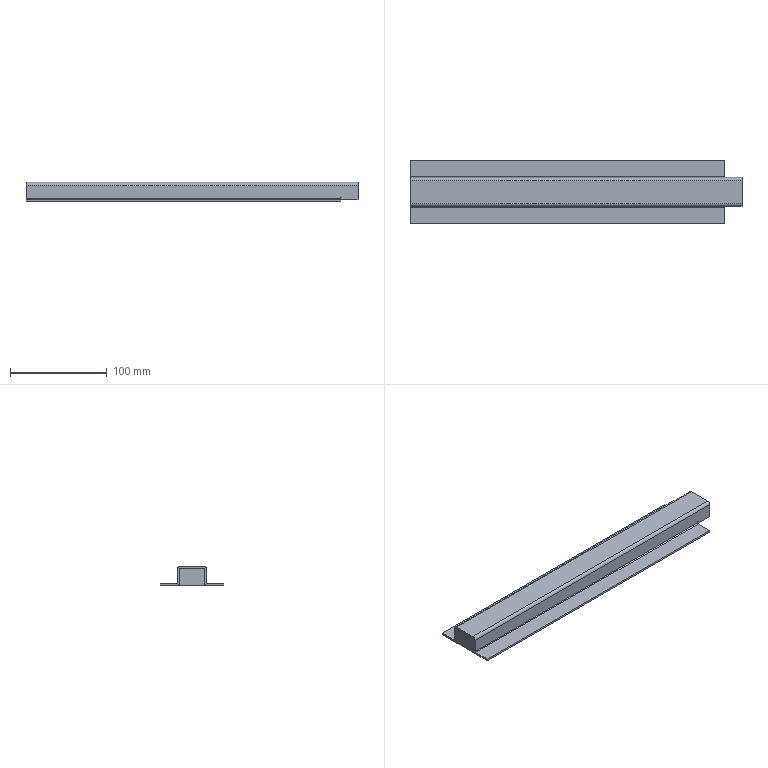Part | SolidWorks | features BaseBody 2 | 2 solids | 56 faces | box 343.5 x 66 x 20 mm | volume 67264 mm3 | plane 46 | cylinder 10 | commonest cylinder face diameters 2 x6 6 x4
STEP:
#1=CARTESIAN_POINT('',(154.75,15.,-18.));
#2=VERTEX_POINT('',#1);
#3=CARTESIAN_POINT('',(171.75,15.,-18.));
#4=VERTEX_POINT('',#3);
#5=CARTESIAN_POINT('',(0.,15.,-18.));
#6=DIRECTION('',(1.,0.,0.));
#7=VECTOR('',#6,1000.);
#8=LINE('',#5,#7);
#9=EDGE_CURVE('',#2,#4,#8,.T.);
#10=ORIENTED_EDGE('',*,*,#9,.T.);
#11=CARTESIAN_POINT('',(171.75,13.,-18.));
#12=VERTEX_POINT('',#11);
#13=CARTESIAN_POINT('',(171.75,33.,-18.));
#14=DIRECTION('',(0.,-1.,0.));
#15=VECTOR('',#14,1000.);
#16=LINE('',#13,#15);
#17=EDGE_CURVE('',#4,#12,#16,.T.);
#18=ORIENTED_EDGE('',*,*,#17,.T.);
#19=CARTESIAN_POINT('',(154.75,13.,-18.));
#20=VERTEX_POINT('',#19);
#21=CARTESIAN_POINT('',(0.,13.,-18.));
#22=DIRECTION('',(1.,0.,0.));
#23=VECTOR('',#22,1000.);
#24=LINE('',#21,#23);
#25=EDGE_CURVE('',#20,#12,#24,.T.);
#26=ORIENTED_EDGE('',*,*,#25,.F.);
#27=CARTESIAN_POINT('',(154.75,15.,-18.));
#28=DIRECTION('',(0.,1.,0.));
#29=VECTOR('',#28,1000.);
#30=LINE('',#27,#29);
#31=EDGE_CURVE('',#20,#2,#30,.T.);
#32=ORIENTED_EDGE('',*,*,#31,.T.);
#33=EDGE_LOOP('',(#10,#18,#26,#32));
#34=FACE_OUTER_BOUND('',#33,.T.);
#35=CARTESIAN_POINT('',(171.75,33.,-18.));
#36=DIRECTION('',(0.,0.,1.));
#37=DIRECTION('',(0.,-1.,0.));
#38=AXIS2_PLACEMENT_3D('',#35,#36,#37);
#39=PLANE('',#38);
#40=ADVANCED_FACE('',(#34),#39,.F.);
#41=CARTESIAN_POINT('',(154.75,-13.,-18.));
#42=VERTEX_POINT('',#41);
#43=CARTESIAN_POINT('',(171.75,-13.,-18.));
#44=VERTEX_POINT('',#43);
#45=CARTESIAN_POINT('',(0.,-13.,-18.));
#46=DIRECTION('',(1.,0.,0.));
#47=VECTOR('',#46,1000.);
#48=LINE('',#45,#47);
#49=EDGE_CURVE('',#42,#44,#48,.T.);
#50=ORIENTED_EDGE('',*,*,#49,.T.);
#51=CARTESIAN_POINT('',(171.75,-15.,-18.));
#52=VERTEX_POINT('',#51);
#53=CARTESIAN_POINT('',(171.75,33.,-18.));
#54=DIRECTION('',(0.,-1.,0.));
#55=VECTOR('',#54,1000.);
#56=LINE('',#53,#55);
#57=EDGE_CURVE('',#44,#52,#56,.T.);
#58=ORIENTED_EDGE('',*,*,#57,.T.);
#59=CARTESIAN_POINT('',(154.75,-15.,-18.));
#60=VERTEX_POINT('',#59);
#61=CARTESIAN_POINT('',(171.75,-15.,-18.));
#62=DIRECTION('',(-1.,0.,0.));
#63=VECTOR('',#62,1000.);
#64=LINE('',#61,#63);
#65=EDGE_CURVE('',#52,#60,#64,.T.);
#66=ORIENTED_EDGE('',*,*,#65,.T.);
#67=CARTESIAN_POINT('',(154.75,-15.,-18.));
#68=DIRECTION('',(0.,1.,0.));
#69=VECTOR('',#68,1000.);
#70=LINE('',#67,#69);
#71=EDGE_CURVE('',#60,#42,#70,.T.);
#72=ORIENTED_EDGE('',*,*,#71,.T.);
#73=EDGE_LOOP('',(#50,#58,#66,#72));
#74=FACE_OUTER_BOUND('',#73,.T.);
#75=CARTESIAN_POINT('',(171.75,33.,-18.));
#76=DIRECTION('',(0.,0.,1.));
#77=DIRECTION('',(0.,-1.,0.));
#78=AXIS2_PLACEMENT_3D('',#75,#76,#77);
#79=PLANE('',#78);
#80=ADVANCED_FACE('',(#74),#79,.F.);
#81=CARTESIAN_POINT('',(-171.75,-33.,-18.));
#82=VERTEX_POINT('',#81);
#83=CARTESIAN_POINT('',(153.75,-33.,-18.));
#84=VERTEX_POINT('',#83);
#85=CARTESIAN_POINT('',(0.,-33.,-18.));
#86=DIRECTION('',(1.,0.,0.));
#87=VECTOR('',#86,1000.);
#88=LINE('',#85,#87);
#89=EDGE_CURVE('',#82,#84,#88,.T.);
#90=ORIENTED_EDGE('',*,*,#89,.F.);
#91=CARTESIAN_POINT('',(-171.75,-33.,-20.));
#92=VERTEX_POINT('',#91);
#93=CARTESIAN_POINT('',(-171.75,-33.,-20.));
#94=DIRECTION('',(0.,0.,1.));
#95=VECTOR('',#94,1000.);
#96=LINE('',#93,#95);
#97=EDGE_CURVE('',#92,#82,#96,.T.);
#98=ORIENTED_EDGE('',*,*,#97,.F.);
#99=CARTESIAN_POINT('',(153.75,-33.,-20.));
#100=VERTEX_POINT('',#99);
#101=CARTESIAN_POINT('',(-171.75,-33.,-20.));
#102=DIRECTION('',(1.,0.,0.));
#103=VECTOR('',#102,1000.);
#104=LINE('',#101,#103);
#105=EDGE_CURVE('',#92,#100,#104,.T.);
#106=ORIENTED_EDGE('',*,*,#105,.T.);
#107=CARTESIAN_POINT('',(153.75,-33.,-20.));
#108=DIRECTION('',(0.,0.,1.));
#109=VECTOR('',#108,1000.);
#110=LINE('',#107,#109);
#111=EDGE_CURVE('',#100,#84,#110,.T.);
#112=ORIENTED_EDGE('',*,*,#111,.T.);
#113=EDGE_LOOP('',(#90,#98,#106,#112));
#114=FACE_OUTER_BOUND('',#113,.T.);
#115=CARTESIAN_POINT('',(-171.75,-33.,-20.));
#116=DIRECTION('',(0.,-1.,0.));
#117=DIRECTION('',(0.,0.,-1.));
#118=AXIS2_PLACEMENT_3D('',#115,#116,#117);
#119=PLANE('',#118);
#120=ADVANCED_FACE('',(#114),#119,.T.);
#121=CARTESIAN_POINT('',(153.75,-16.,-18.));
#122=VERTEX_POINT('',#121);
#123=CARTESIAN_POINT('',(153.75,0.,-18.));
#124=DIRECTION('',(0.,1.,0.));
#125=VECTOR('',#124,1000.);
#126=LINE('',#123,#125);
#127=EDGE_CURVE('',#84,#122,#126,.T.);
#128=ORIENTED_EDGE('',*,*,#127,.T.);
#129=CARTESIAN_POINT('',(-171.75,-16.,-18.));
#130=VERTEX_POINT('',#129);
#131=CARTESIAN_POINT('',(-171.75,-16.,-18.));
#132=DIRECTION('',(1.,0.,0.));
#133=VECTOR('',#132,1000.);
#134=LINE('',#131,#133);
#135=EDGE_CURVE('',#130,#122,#134,.T.);
#136=ORIENTED_EDGE('',*,*,#135,.F.);
#137=CARTESIAN_POINT('',(-171.75,0.,-18.));
#138=DIRECTION('',(0.,-1.,0.));
#139=VECTOR('',#138,1000.);
#140=LINE('',#137,#139);
#141=EDGE_CURVE('',#130,#82,#140,.T.);
#142=ORIENTED_EDGE('',*,*,#141,.T.);
#143=ORIENTED_EDGE('',*,*,#89,.T.);
#144=EDGE_LOOP('',(#128,#136,#142,#143));
#145=FACE_OUTER_BOUND('',#144,.T.);
#146=CARTESIAN_POINT('',(0.,0.,-18.));
#147=DIRECTION('',(0.,0.,1.));
#148=DIRECTION('',(1.,0.,0.));
#149=AXIS2_PLACEMENT_3D('',#146,#147,#148);
#150=PLANE('',#149);
#151=ADVANCED_FACE('',(#145),#150,.T.);
#152=CARTESIAN_POINT('',(153.75,-16.,-20.));
#153=VERTEX_POINT('',#152);
#154=CARTESIAN_POINT('',(-171.75,-16.,-20.));
#155=VERTEX_POINT('',#154);
#156=CARTESIAN_POINT('',(-171.75,-16.,-20.));
#157=DIRECTION('',(-1.,0.,0.));
#158=VECTOR('',#157,1000.);
#159=LINE('',#156,#158);
#160=EDGE_CURVE('',#153,#155,#159,.T.);
#161=ORIENTED_EDGE('',*,*,#160,.F.);
#162=CARTESIAN_POINT('',(153.75,-33.,-20.));
#163=DIRECTION('',(0.,1.,0.));
#164=VECTOR('',#163,1000.);
#165=LINE('',#162,#164);
#166=EDGE_CURVE('',#100,#153,#165,.T.);
#167=ORIENTED_EDGE('',*,*,#166,.F.);
#168=ORIENTED_EDGE('',*,*,#105,.F.);
#169=CARTESIAN_POINT('',(-171.75,-15.,-20.));
#170=DIRECTION('',(0.,-1.,0.));
#171=VECTOR('',#170,1000.);
#172=LINE('',#169,#171);
#173=EDGE_CURVE('',#155,#92,#172,.T.);
#174=ORIENTED_EDGE('',*,*,#173,.F.);
#175=EDGE_LOOP('',(#161,#167,#168,#174));
#176=FACE_OUTER_BOUND('',#175,.T.);
#177=CARTESIAN_POINT('',(0.,0.,-20.));
#178=DIRECTION('',(0.,0.,1.));
#179=DIRECTION('',(1.,0.,0.));
#180=AXIS2_PLACEMENT_3D('',#177,#178,#179);
#181=PLANE('',#180);
#182=ADVANCED_FACE('',(#176),#181,.F.);
#183=ORIENTED_EDGE('',*,*,#166,.T.);
#184=CARTESIAN_POINT('',(153.75,-16.,-18.));
#185=DIRECTION('',(0.,0.,-1.));
#186=VECTOR('',#185,1000.);
#187=LINE('',#184,#186);
#188=EDGE_CURVE('',#122,#153,#187,.T.);
#189=ORIENTED_EDGE('',*,*,#188,.F.);
#190=ORIENTED_EDGE('',*,*,#127,.F.);
#191=ORIENTED_EDGE('',*,*,#111,.F.);
#192=EDGE_LOOP('',(#183,#189,#190,#191));
#193=FACE_OUTER_BOUND('',#192,.T.);
#194=CARTESIAN_POINT('',(153.75,-33.,-20.));
#195=DIRECTION('',(1.,0.,0.));
#196=DIRECTION('',(0.,0.,-1.));
#197=AXIS2_PLACEMENT_3D('',#194,#195,#196);
#198=PLANE('',#197);
#199=ADVANCED_FACE('',(#193),#198,.T.);
#200=ORIENTED_EDGE('',*,*,#141,.F.);
#201=CARTESIAN_POINT('',(-171.75,-16.,-20.));
#202=DIRECTION('',(0.,0.,-1.));
#203=VECTOR('',#202,1000.);
#204=LINE('',#201,#203);
#205=EDGE_CURVE('',#130,#155,#204,.T.);
#206=ORIENTED_EDGE('',*,*,#205,.T.);
#207=ORIENTED_EDGE('',*,*,#173,.T.);
#208=ORIENTED_EDGE('',*,*,#97,.T.);
#209=EDGE_LOOP('',(#200,#206,#207,#208));
#210=FACE_OUTER_BOUND('',#209,.T.);
#211=CARTESIAN_POINT('',(-171.75,-15.,-20.));
#212=DIRECTION('',(-1.,0.,0.));
#213=DIRECTION('',(0.,1.,0.));
#214=AXIS2_PLACEMENT_3D('',#211,#212,#213);
#215=PLANE('',#214);
#216=ADVANCED_FACE('',(#210),#215,.T.);
#217=CARTESIAN_POINT('',(153.75,-15.,-17.));
#218=VERTEX_POINT('',#217);
#219=CARTESIAN_POINT('',(-171.75,-15.,-17.));
#220=VERTEX_POINT('',#219);
#221=CARTESIAN_POINT('',(153.75,-15.,-17.));
#222=DIRECTION('',(-1.,0.,0.));
#223=VECTOR('',#222,1000.);
#224=LINE('',#221,#223);
#225=EDGE_CURVE('',#218,#220,#224,.T.);
#226=ORIENTED_EDGE('',*,*,#225,.T.);
#227=CARTESIAN_POINT('',(-171.75,-16.,-17.));
#228=DIRECTION('',(-1.,0.,0.));
#229=DIRECTION('',(0.,0.,-1.));
#230=AXIS2_PLACEMENT_3D('',#227,#228,#229);
#231=CIRCLE('',#230,1.);
#232=EDGE_CURVE('',#220,#130,#231,.T.);
#233=ORIENTED_EDGE('',*,*,#232,.T.);
#234=ORIENTED_EDGE('',*,*,#135,.T.);
#235=CARTESIAN_POINT('',(153.75,-16.,-17.));
#236=DIRECTION('',(1.,0.,0.));
#237=DIRECTION('',(0.,0.,-1.));
#238=AXIS2_PLACEMENT_3D('',#235,#236,#237);
#239=CIRCLE('',#238,1.);
#240=EDGE_CURVE('',#122,#218,#239,.T.);
#241=ORIENTED_EDGE('',*,*,#240,.T.);
#242=EDGE_LOOP('',(#226,#233,#234,#241));
#243=FACE_OUTER_BOUND('',#242,.T.);
#244=CARTESIAN_POINT('',(153.75,-16.,-17.));
#245=DIRECTION('',(1.,0.,0.));
#246=DIRECTION('',(0.,0.,-1.));
#247=AXIS2_PLACEMENT_3D('',#244,#245,#246);
#248=CYLINDRICAL_SURFACE('',#247,1.);
#249=ADVANCED_FACE('',(#243),#248,.F.);
#250=CARTESIAN_POINT('',(153.75,-13.,-17.));
#251=VERTEX_POINT('',#250);
#252=CARTESIAN_POINT('',(-171.75,-13.,-17.));
#253=VERTEX_POINT('',#252);
#254=CARTESIAN_POINT('',(153.75,-13.,-17.));
#255=DIRECTION('',(-1.,0.,0.));
#256=VECTOR('',#255,1000.);
#257=LINE('',#254,#256);
#258=EDGE_CURVE('',#251,#253,#257,.T.);
#259=ORIENTED_EDGE('',*,*,#258,.F.);
#260=CARTESIAN_POINT('',(153.75,-13.172,-18.));
#261=VERTEX_POINT('',#260);
#262=CARTESIAN_POINT('',(153.75,-16.,-17.));
#263=DIRECTION('',(1.,0.,0.));
#264=DIRECTION('',(0.,0.,-1.));
#265=AXIS2_PLACEMENT_3D('',#262,#263,#264);
#266=CIRCLE('',#265,3.);
#267=EDGE_CURVE('',#261,#251,#266,.T.);
#268=ORIENTED_EDGE('',*,*,#267,.F.);
#269=CARTESIAN_POINT('',(153.75,-15.,-19.828));
#270=VERTEX_POINT('',#269);
#271=CARTESIAN_POINT('',(153.75,-16.,-17.));
#272=DIRECTION('',(1.,0.,0.));
#273=DIRECTION('',(0.,0.,-1.));
#274=AXIS2_PLACEMENT_3D('',#271,#272,#273);
#275=CIRCLE('',#274,3.);
#276=EDGE_CURVE('',#270,#261,#275,.T.);
#277=ORIENTED_EDGE('',*,*,#276,.F.);
#278=CARTESIAN_POINT('',(153.75,-16.,-17.));
#279=DIRECTION('',(1.,0.,0.));
#280=DIRECTION('',(0.,0.,-1.));
#281=AXIS2_PLACEMENT_3D('',#278,#279,#280);
#282=CIRCLE('',#281,3.);
#283=EDGE_CURVE('',#153,#270,#282,.T.);
#284=ORIENTED_EDGE('',*,*,#283,.F.);
#285=ORIENTED_EDGE('',*,*,#160,.T.);
#286=CARTESIAN_POINT('',(-171.75,-16.,-17.));
#287=DIRECTION('',(-1.,0.,0.));
#288=DIRECTION('',(0.,0.,-1.));
#289=AXIS2_PLACEMENT_3D('',#286,#287,#288);
#290=CIRCLE('',#289,3.);
#291=EDGE_CURVE('',#253,#155,#290,.T.);
#292=ORIENTED_EDGE('',*,*,#291,.F.);
#293=EDGE_LOOP('',(#259,#268,#277,#284,#285,#292));
#294=FACE_OUTER_BOUND('',#293,.T.);
#295=CARTESIAN_POINT('',(153.75,-16.,-17.));
#296=DIRECTION('',(1.,0.,0.));
#297=DIRECTION('',(0.,0.,-1.));
#298=AXIS2_PLACEMENT_3D('',#295,#296,#297);
#299=CYLINDRICAL_SURFACE('',#298,3.);
#300=ADVANCED_FACE('',(#294),#299,.T.);
#301=CARTESIAN_POINT('',(153.75,-15.,-18.));
#302=VERTEX_POINT('',#301);
#303=CARTESIAN_POINT('',(153.75,-16.,-18.));
#304=DIRECTION('',(0.,-1.,0.));
#305=VECTOR('',#304,1000.);
#306=LINE('',#303,#305);
#307=EDGE_CURVE('',#261,#302,#306,.T.);
#308=ORIENTED_EDGE('',*,*,#307,.F.);
#309=ORIENTED_EDGE('',*,*,#267,.T.);
#310=CARTESIAN_POINT('',(153.75,-15.,-17.));
#311=DIRECTION('',(0.,1.,0.));
#312=VECTOR('',#311,1000.);
#313=LINE('',#310,#312);
#314=EDGE_CURVE('',#218,#251,#313,.T.);
#315=ORIENTED_EDGE('',*,*,#314,.F.);
#316=ORIENTED_EDGE('',*,*,#240,.F.);
#317=ORIENTED_EDGE('',*,*,#188,.T.);
#318=ORIENTED_EDGE('',*,*,#283,.T.);
#319=CARTESIAN_POINT('',(153.75,-15.,-17.));
#320=DIRECTION('',(0.,0.,-1.));
#321=VECTOR('',#320,1000.);
#322=LINE('',#319,#321);
#323=EDGE_CURVE('',#302,#270,#322,.T.);
#324=ORIENTED_EDGE('',*,*,#323,.F.);
#325=EDGE_LOOP('',(#308,#309,#315,#316,#317,#318,#324));
#326=FACE_OUTER_BOUND('',#325,.T.);
#327=CARTESIAN_POINT('',(153.75,-16.,-17.));
#328=DIRECTION('',(-1.,0.,0.));
#329=DIRECTION('',(0.,0.,1.));
#330=AXIS2_PLACEMENT_3D('',#327,#328,#329);
#331=PLANE('',#330);
#332=ADVANCED_FACE('',(#326),#331,.F.);
#333=ORIENTED_EDGE('',*,*,#205,.F.);
#334=ORIENTED_EDGE('',*,*,#232,.F.);
#335=CARTESIAN_POINT('',(-171.75,-15.,-17.));
#336=DIRECTION('',(0.,1.,0.));
#337=VECTOR('',#336,1000.);
#338=LINE('',#335,#337);
#339=EDGE_CURVE('',#220,#253,#338,.T.);
#340=ORIENTED_EDGE('',*,*,#339,.T.);
#341=ORIENTED_EDGE('',*,*,#291,.T.);
#342=EDGE_LOOP('',(#333,#334,#340,#341));
#343=FACE_OUTER_BOUND('',#342,.T.);
#344=CARTESIAN_POINT('',(-171.75,-16.,-17.));
#345=DIRECTION('',(-1.,0.,0.));
#346=DIRECTION('',(0.,0.,1.));
#347=AXIS2_PLACEMENT_3D('',#344,#345,#346);
#348=PLANE('',#347);
#349=ADVANCED_FACE('',(#343),#348,.T.);
#350=CARTESIAN_POINT('',(153.75,33.,-18.));
#351=VERTEX_POINT('',#350);
#352=CARTESIAN_POINT('',(-171.75,33.,-18.));
#353=VERTEX_POINT('',#352);
#354=CARTESIAN_POINT('',(0.,33.,-18.));
#355=DIRECTION('',(-1.,0.,0.));
#356=VECTOR('',#355,1000.);
#357=LINE('',#354,#356);
#358=EDGE_CURVE('',#351,#353,#357,.T.);
#359=ORIENTED_EDGE('',*,*,#358,.F.);
#360=CARTESIAN_POINT('',(153.75,33.,-20.));
#361=VERTEX_POINT('',#360);
#362=CARTESIAN_POINT('',(153.75,33.,-20.));
#363=DIRECTION('',(0.,0.,1.));
#364=VECTOR('',#363,1000.);
#365=LINE('',#362,#364);
#366=EDGE_CURVE('',#361,#351,#365,.T.);
#367=ORIENTED_EDGE('',*,*,#366,.F.);
#368=CARTESIAN_POINT('',(-171.75,33.,-20.));
#369=VERTEX_POINT('',#368);
#370=CARTESIAN_POINT('',(-171.75,33.,-20.));
#371=DIRECTION('',(-1.,0.,0.));
#372=VECTOR('',#371,1000.);
#373=LINE('',#370,#372);
#374=EDGE_CURVE('',#361,#369,#373,.T.);
#375=ORIENTED_EDGE('',*,*,#374,.T.);
#376=CARTESIAN_POINT('',(-171.75,33.,-20.));
#377=DIRECTION('',(0.,0.,1.));
#378=VECTOR('',#377,1000.);
#379=LINE('',#376,#378);
#380=EDGE_CURVE('',#369,#353,#379,.T.);
#381=ORIENTED_EDGE('',*,*,#380,.T.);
#382=EDGE_LOOP('',(#359,#367,#375,#381));
#383=FACE_OUTER_BOUND('',#382,.T.);
#384=CARTESIAN_POINT('',(-171.75,33.,-20.));
#385=DIRECTION('',(0.,1.,0.));
#386=DIRECTION('',(1.,0.,0.));
#387=AXIS2_PLACEMENT_3D('',#384,#385,#386);
#388=PLANE('',#387);
#389=ADVANCED_FACE('',(#383),#388,.T.);
#390=CARTESIAN_POINT('',(153.75,16.,-18.));
#391=VERTEX_POINT('',#390);
#392=CARTESIAN_POINT('',(-171.75,16.,-18.));
#393=VERTEX_POINT('',#392);
#394=CARTESIAN_POINT('',(153.75,16.,-18.));
#395=DIRECTION('',(-1.,0.,0.));
#396=VECTOR('',#395,1000.);
#397=LINE('',#394,#396);
#398=EDGE_CURVE('',#391,#393,#397,.T.);
#399=ORIENTED_EDGE('',*,*,#398,.F.);
#400=CARTESIAN_POINT('',(153.75,0.,-18.));
#401=DIRECTION('',(0.,1.,0.));
#402=VECTOR('',#401,1000.);
#403=LINE('',#400,#402);
#404=EDGE_CURVE('',#391,#351,#403,.T.);
#405=ORIENTED_EDGE('',*,*,#404,.T.);
#406=ORIENTED_EDGE('',*,*,#358,.T.);
#407=CARTESIAN_POINT('',(-171.75,0.,-18.));
#408=DIRECTION('',(0.,-1.,0.));
#409=VECTOR('',#408,1000.);
#410=LINE('',#407,#409);
#411=EDGE_CURVE('',#353,#393,#410,.T.);
#412=ORIENTED_EDGE('',*,*,#411,.T.);
#413=EDGE_LOOP('',(#399,#405,#406,#412));
#414=FACE_OUTER_BOUND('',#413,.T.);
#415=CARTESIAN_POINT('',(0.,0.,-18.));
#416=DIRECTION('',(0.,0.,-1.));
#417=DIRECTION('',(0.,-1.,0.));
#418=AXIS2_PLACEMENT_3D('',#415,#416,#417);
#419=PLANE('',#418);
#420=ADVANCED_FACE('',(#414),#419,.F.);
#421=CARTESIAN_POINT('',(153.75,16.,-20.));
#422=VERTEX_POINT('',#421);
#423=CARTESIAN_POINT('',(153.75,15.,-20.));
#424=DIRECTION('',(0.,1.,0.));
#425=VECTOR('',#424,1000.);
#426=LINE('',#423,#425);
#427=EDGE_CURVE('',#422,#361,#426,.T.);
#428=ORIENTED_EDGE('',*,*,#427,.F.);
#429=CARTESIAN_POINT('',(-171.75,16.,-20.));
#430=VERTEX_POINT('',#429);
#431=CARTESIAN_POINT('',(0.,16.,-20.));
#432=DIRECTION('',(-1.,0.,0.));
#433=VECTOR('',#432,1000.);
#434=LINE('',#431,#433);
#435=EDGE_CURVE('',#422,#430,#434,.T.);
#436=ORIENTED_EDGE('',*,*,#435,.T.);
#437=CARTESIAN_POINT('',(-171.75,15.,-20.));
#438=DIRECTION('',(0.,-1.,0.));
#439=VECTOR('',#438,1000.);
#440=LINE('',#437,#439);
#441=EDGE_CURVE('',#369,#430,#440,.T.);
#442=ORIENTED_EDGE('',*,*,#441,.F.);
#443=ORIENTED_EDGE('',*,*,#374,.F.);
#444=EDGE_LOOP('',(#428,#436,#442,#443));
#445=FACE_OUTER_BOUND('',#444,.T.);
#446=CARTESIAN_POINT('',(0.,0.,-20.));
#447=DIRECTION('',(0.,0.,-1.));
#448=DIRECTION('',(0.,-1.,0.));
#449=AXIS2_PLACEMENT_3D('',#446,#447,#448);
#450=PLANE('',#449);
#451=ADVANCED_FACE('',(#445),#450,.T.);
#452=ORIENTED_EDGE('',*,*,#441,.T.);
#453=CARTESIAN_POINT('',(-171.75,16.,-18.));
#454=DIRECTION('',(0.,0.,-1.));
#455=VECTOR('',#454,1000.);
#456=LINE('',#453,#455);
#457=EDGE_CURVE('',#393,#430,#456,.T.);
#458=ORIENTED_EDGE('',*,*,#457,.F.);
#459=ORIENTED_EDGE('',*,*,#411,.F.);
#460=ORIENTED_EDGE('',*,*,#380,.F.);
#461=EDGE_LOOP('',(#452,#458,#459,#460));
#462=FACE_OUTER_BOUND('',#461,.T.);
#463=CARTESIAN_POINT('',(-171.75,15.,-20.));
#464=DIRECTION('',(-1.,0.,0.));
#465=DIRECTION('',(0.,0.,1.));
#466=AXIS2_PLACEMENT_3D('',#463,#464,#465);
#467=PLANE('',#466);
#468=ADVANCED_FACE('',(#462),#467,.T.);
#469=ORIENTED_EDGE('',*,*,#404,.F.);
#470=CARTESIAN_POINT('',(153.75,16.,-20.));
#471=DIRECTION('',(0.,0.,-1.));
#472=VECTOR('',#471,1000.);
#473=LINE('',#470,#472);
#474=EDGE_CURVE('',#391,#422,#473,.T.);
#475=ORIENTED_EDGE('',*,*,#474,.T.);
#476=ORIENTED_EDGE('',*,*,#427,.T.);
#477=ORIENTED_EDGE('',*,*,#366,.T.);
#478=EDGE_LOOP('',(#469,#475,#476,#477));
#479=FACE_OUTER_BOUND('',#478,.T.);
#480=CARTESIAN_POINT('',(153.75,15.,-20.));
#481=DIRECTION('',(1.,0.,0.));
#482=DIRECTION('',(0.,1.,0.));
#483=AXIS2_PLACEMENT_3D('',#480,#481,#482);
#484=PLANE('',#483);
#485=ADVANCED_FACE('',(#479),#484,.T.);
#486=CARTESIAN_POINT('',(-171.75,15.,-17.));
#487=VERTEX_POINT('',#486);
#488=CARTESIAN_POINT('',(153.75,15.,-17.));
#489=VERTEX_POINT('',#488);
#490=CARTESIAN_POINT('',(-171.75,15.,-17.));
#491=DIRECTION('',(1.,0.,0.));
#492=VECTOR('',#491,1000.);
#493=LINE('',#490,#492);
#494=EDGE_CURVE('',#487,#489,#493,.T.);
#495=ORIENTED_EDGE('',*,*,#494,.T.);
#496=CARTESIAN_POINT('',(153.75,16.,-17.));
#497=DIRECTION('',(1.,0.,0.));
#498=DIRECTION('',(0.,0.,1.));
#499=AXIS2_PLACEMENT_3D('',#496,#497,#498);
#500=CIRCLE('',#499,1.);
#501=EDGE_CURVE('',#489,#391,#500,.T.);
#502=ORIENTED_EDGE('',*,*,#501,.T.);
#503=ORIENTED_EDGE('',*,*,#398,.T.);
#504=CARTESIAN_POINT('',(-171.75,16.,-17.));
#505=DIRECTION('',(-1.,0.,0.));
#506=DIRECTION('',(0.,0.,1.));
#507=AXIS2_PLACEMENT_3D('',#504,#505,#506);
#508=CIRCLE('',#507,1.);
#509=EDGE_CURVE('',#393,#487,#508,.T.);
#510=ORIENTED_EDGE('',*,*,#509,.T.);
#511=EDGE_LOOP('',(#495,#502,#503,#510));
#512=FACE_OUTER_BOUND('',#511,.T.);
#513=CARTESIAN_POINT('',(-171.75,16.,-17.));
#514=DIRECTION('',(-1.,0.,0.));
#515=DIRECTION('',(0.,0.,-1.));
#516=AXIS2_PLACEMENT_3D('',#513,#514,#515);
#517=CYLINDRICAL_SURFACE('',#516,1.);
#518=ADVANCED_FACE('',(#512),#517,.F.);
#519=CARTESIAN_POINT('',(-171.75,13.,-17.));
#520=VERTEX_POINT('',#519);
#521=CARTESIAN_POINT('',(153.75,13.,-17.));
#522=VERTEX_POINT('',#521);
#523=CARTESIAN_POINT('',(-171.75,13.,-17.));
#524=DIRECTION('',(1.,0.,0.));
#525=VECTOR('',#524,1000.);
#526=LINE('',#523,#525);
#527=EDGE_CURVE('',#520,#522,#526,.T.);
#528=ORIENTED_EDGE('',*,*,#527,.F.);
#529=CARTESIAN_POINT('',(-171.75,16.,-17.));
#530=DIRECTION('',(-1.,0.,0.));
#531=DIRECTION('',(0.,0.,1.));
#532=AXIS2_PLACEMENT_3D('',#529,#530,#531);
#533=CIRCLE('',#532,3.);
#534=EDGE_CURVE('',#430,#520,#533,.T.);
#535=ORIENTED_EDGE('',*,*,#534,.F.);
#536=ORIENTED_EDGE('',*,*,#435,.F.);
#537=CARTESIAN_POINT('',(153.75,13.172,-18.));
#538=VERTEX_POINT('',#537);
#539=CARTESIAN_POINT('',(153.75,16.,-17.));
#540=DIRECTION('',(1.,0.,0.));
#541=DIRECTION('',(0.,0.,1.));
#542=AXIS2_PLACEMENT_3D('',#539,#540,#541);
#543=CIRCLE('',#542,3.);
#544=EDGE_CURVE('',#538,#422,#543,.T.);
#545=ORIENTED_EDGE('',*,*,#544,.F.);
#546=CARTESIAN_POINT('',(153.75,16.,-17.));
#547=DIRECTION('',(1.,0.,0.));
#548=DIRECTION('',(0.,0.,1.));
#549=AXIS2_PLACEMENT_3D('',#546,#547,#548);
#550=CIRCLE('',#549,3.);
#551=EDGE_CURVE('',#522,#538,#550,.T.);
#552=ORIENTED_EDGE('',*,*,#551,.F.);
#553=EDGE_LOOP('',(#528,#535,#536,#545,#552));
#554=FACE_OUTER_BOUND('',#553,.T.);
#555=CARTESIAN_POINT('',(-171.75,16.,-17.));
#556=DIRECTION('',(-1.,0.,0.));
#557=DIRECTION('',(0.,0.,-1.));
#558=AXIS2_PLACEMENT_3D('',#555,#556,#557);
#559=CYLINDRICAL_SURFACE('',#558,3.);
#560=ADVANCED_FACE('',(#554),#559,.T.);
#561=ORIENTED_EDGE('',*,*,#509,.F.);
#562=ORIENTED_EDGE('',*,*,#457,.T.);
#563=ORIENTED_EDGE('',*,*,#534,.T.);
#564=CARTESIAN_POINT('',(-171.75,15.,-17.));
#565=DIRECTION('',(0.,-1.,0.));
#566=VECTOR('',#565,1000.);
#567=LINE('',#564,#566);
#568=EDGE_CURVE('',#487,#520,#567,.T.);
#569=ORIENTED_EDGE('',*,*,#568,.F.);
#570=EDGE_LOOP('',(#561,#562,#563,#569));
#571=FACE_OUTER_BOUND('',#570,.T.);
#572=CARTESIAN_POINT('',(-171.75,16.,-17.));
#573=DIRECTION('',(1.,0.,0.));
#574=DIRECTION('',(0.,1.,0.));
#575=AXIS2_PLACEMENT_3D('',#572,#573,#574);
#576=PLANE('',#575);
#577=ADVANCED_FACE('',(#571),#576,.F.);
#578=CARTESIAN_POINT('',(153.75,16.,-18.));
#579=DIRECTION('',(0.,-1.,0.));
#580=VECTOR('',#579,1000.);
#581=LINE('',#578,#580);
#582=EDGE_CURVE('',#391,#538,#581,.T.);
#583=ORIENTED_EDGE('',*,*,#582,.F.);
#584=ORIENTED_EDGE('',*,*,#501,.F.);
#585=CARTESIAN_POINT('',(153.75,15.,-17.));
#586=DIRECTION('',(0.,-1.,0.));
#587=VECTOR('',#586,1000.);
#588=LINE('',#585,#587);
#589=EDGE_CURVE('',#489,#522,#588,.T.);
#590=ORIENTED_EDGE('',*,*,#589,.T.);
#591=ORIENTED_EDGE('',*,*,#551,.T.);
#592=EDGE_LOOP('',(#583,#584,#590,#591));
#593=FACE_OUTER_BOUND('',#592,.T.);
#594=CARTESIAN_POINT('',(153.75,16.,-17.));
#595=DIRECTION('',(1.,0.,0.));
#596=DIRECTION('',(0.,1.,0.));
#597=AXIS2_PLACEMENT_3D('',#594,#595,#596);
#598=PLANE('',#597);
#599=ADVANCED_FACE('',(#593),#598,.T.);
#600=CARTESIAN_POINT('',(153.75,-13.,-16.));
#601=VERTEX_POINT('',#600);
#602=CARTESIAN_POINT('',(153.75,-13.,0.));
#603=DIRECTION('',(0.,0.,-1.));
#604=VECTOR('',#603,1000.);
#605=LINE('',#602,#604);
#606=EDGE_CURVE('',#601,#251,#605,.T.);
#607=ORIENTED_EDGE('',*,*,#606,.F.);
#608=CARTESIAN_POINT('',(153.75,-15.,-16.));
#609=VERTEX_POINT('',#608);
#610=CARTESIAN_POINT('',(153.75,-15.,-16.));
#611=DIRECTION('',(0.,1.,0.));
#612=VECTOR('',#611,1000.);
#613=LINE('',#610,#612);
#614=EDGE_CURVE('',#609,#601,#613,.T.);
#615=ORIENTED_EDGE('',*,*,#614,.F.);
#616=CARTESIAN_POINT('',(153.75,-15.,-16.));
#617=DIRECTION('',(0.,0.,-1.));
#618=VECTOR('',#617,1000.);
#619=LINE('',#616,#618);
#620=EDGE_CURVE('',#609,#218,#619,.T.);
#621=ORIENTED_EDGE('',*,*,#620,.T.);
#622=ORIENTED_EDGE('',*,*,#314,.T.);
#623=EDGE_LOOP('',(#607,#615,#621,#622));
#624=FACE_OUTER_BOUND('',#623,.T.);
#625=CARTESIAN_POINT('',(153.75,-15.,-16.));
#626=DIRECTION('',(1.,0.,0.));
#627=DIRECTION('',(0.,1.,0.));
#628=AXIS2_PLACEMENT_3D('',#625,#626,#627);
#629=PLANE('',#628);
#630=ADVANCED_FACE('',(#624),#629,.T.);
#631=CARTESIAN_POINT('',(154.75,-13.,-16.));
#632=VERTEX_POINT('',#631);
#633=CARTESIAN_POINT('',(0.,-13.,-16.));
#634=DIRECTION('',(-1.,0.,0.));
#635=VECTOR('',#634,1000.);
#636=LINE('',#633,#635);
#637=EDGE_CURVE('',#632,#601,#636,.T.);
#638=ORIENTED_EDGE('',*,*,#637,.F.);
#639=CARTESIAN_POINT('',(154.75,-15.,-16.));
#640=VERTEX_POINT('',#639);
#641=CARTESIAN_POINT('',(154.75,-15.,-16.));
#642=DIRECTION('',(0.,1.,0.));
#643=VECTOR('',#642,1000.);
#644=LINE('',#641,#643);
#645=EDGE_CURVE('',#640,#632,#644,.T.);
#646=ORIENTED_EDGE('',*,*,#645,.F.);
#647=CARTESIAN_POINT('',(154.75,-15.,-16.));
#648=DIRECTION('',(-1.,0.,0.));
#649=VECTOR('',#648,1000.);
#650=LINE('',#647,#649);
#651=EDGE_CURVE('',#640,#609,#650,.T.);
#652=ORIENTED_EDGE('',*,*,#651,.T.);
#653=ORIENTED_EDGE('',*,*,#614,.T.);
#654=EDGE_LOOP('',(#638,#646,#652,#653));
#655=FACE_OUTER_BOUND('',#654,.T.);
#656=CARTESIAN_POINT('',(154.75,-15.,-16.));
#657=DIRECTION('',(0.,0.,-1.));
#658=DIRECTION('',(0.,-1.,0.));
#659=AXIS2_PLACEMENT_3D('',#656,#657,#658);
#660=PLANE('',#659);
#661=ADVANCED_FACE('',(#655),#660,.T.);
#662=ORIENTED_EDGE('',*,*,#71,.F.);
#663=CARTESIAN_POINT('',(154.75,-15.,-20.));
#664=DIRECTION('',(0.,0.,1.));
#665=VECTOR('',#664,1000.);
#666=LINE('',#663,#665);
#667=EDGE_CURVE('',#60,#640,#666,.T.);
#668=ORIENTED_EDGE('',*,*,#667,.T.);
#669=ORIENTED_EDGE('',*,*,#645,.T.);
#670=CARTESIAN_POINT('',(154.75,-13.,0.));
#671=DIRECTION('',(0.,0.,1.));
#672=VECTOR('',#671,1000.);
#673=LINE('',#670,#672);
#674=EDGE_CURVE('',#42,#632,#673,.T.);
#675=ORIENTED_EDGE('',*,*,#674,.F.);
#676=EDGE_LOOP('',(#662,#668,#669,#675));
#677=FACE_OUTER_BOUND('',#676,.T.);
#678=CARTESIAN_POINT('',(154.75,-15.,-20.));
#679=DIRECTION('',(-1.,0.,0.));
#680=DIRECTION('',(0.,1.,0.));
#681=AXIS2_PLACEMENT_3D('',#678,#679,#680);
#682=PLANE('',#681);
#683=ADVANCED_FACE('',(#677),#682,.T.);
#684=ORIENTED_EDGE('',*,*,#31,.F.);
#685=CARTESIAN_POINT('',(154.75,13.,-16.));
#686=VERTEX_POINT('',#685);
#687=CARTESIAN_POINT('',(154.75,13.,0.));
#688=DIRECTION('',(0.,0.,1.));
#689=VECTOR('',#688,1000.);
#690=LINE('',#687,#689);
#691=EDGE_CURVE('',#20,#686,#690,.T.);
#692=ORIENTED_EDGE('',*,*,#691,.T.);
#693=CARTESIAN_POINT('',(154.75,15.,-16.));
#694=VERTEX_POINT('',#693);
#695=CARTESIAN_POINT('',(154.75,15.,-16.));
#696=DIRECTION('',(0.,-1.,0.));
#697=VECTOR('',#696,1000.);
#698=LINE('',#695,#697);
#699=EDGE_CURVE('',#694,#686,#698,.T.);
#700=ORIENTED_EDGE('',*,*,#699,.F.);
#701=CARTESIAN_POINT('',(154.75,15.,-16.));
#702=DIRECTION('',(0.,0.,-1.));
#703=VECTOR('',#702,1000.);
#704=LINE('',#701,#703);
#705=EDGE_CURVE('',#694,#2,#704,.T.);
#706=ORIENTED_EDGE('',*,*,#705,.T.);
#707=EDGE_LOOP('',(#684,#692,#700,#706));
#708=FACE_OUTER_BOUND('',#707,.T.);
#709=CARTESIAN_POINT('',(154.75,15.,-16.));
#710=DIRECTION('',(-1.,0.,0.));
#711=DIRECTION('',(0.,0.,1.));
#712=AXIS2_PLACEMENT_3D('',#709,#710,#711);
#713=PLANE('',#712);
#714=ADVANCED_FACE('',(#708),#713,.T.);
#715=ORIENTED_EDGE('',*,*,#699,.T.);
#716=CARTESIAN_POINT('',(153.75,13.,-16.));
#717=VERTEX_POINT('',#716);
#718=CARTESIAN_POINT('',(0.,13.,-16.));
#719=DIRECTION('',(-1.,0.,0.));
#720=VECTOR('',#719,1000.);
#721=LINE('',#718,#720);
#722=EDGE_CURVE('',#686,#717,#721,.T.);
#723=ORIENTED_EDGE('',*,*,#722,.T.);
#724=CARTESIAN_POINT('',(153.75,15.,-16.));
#725=VERTEX_POINT('',#724);
#726=CARTESIAN_POINT('',(153.75,15.,-16.));
#727=DIRECTION('',(0.,-1.,0.));
#728=VECTOR('',#727,1000.);
#729=LINE('',#726,#728);
#730=EDGE_CURVE('',#725,#717,#729,.T.);
#731=ORIENTED_EDGE('',*,*,#730,.F.);
#732=CARTESIAN_POINT('',(153.75,15.,-16.));
#733=DIRECTION('',(1.,0.,0.));
#734=VECTOR('',#733,1000.);
#735=LINE('',#732,#734);
#736=EDGE_CURVE('',#725,#694,#735,.T.);
#737=ORIENTED_EDGE('',*,*,#736,.T.);
#738=EDGE_LOOP('',(#715,#723,#731,#737));
#739=FACE_OUTER_BOUND('',#738,.T.);
#740=CARTESIAN_POINT('',(153.75,15.,-16.));
#741=DIRECTION('',(0.,0.,-1.));
#742=DIRECTION('',(-1.,0.,0.));
#743=AXIS2_PLACEMENT_3D('',#740,#741,#742);
#744=PLANE('',#743);
#745=ADVANCED_FACE('',(#739),#744,.T.);
#746=ORIENTED_EDGE('',*,*,#730,.T.);
#747=CARTESIAN_POINT('',(153.75,13.,0.));
#748=DIRECTION('',(0.,0.,-1.));
#749=VECTOR('',#748,1000.);
#750=LINE('',#747,#749);
#751=EDGE_CURVE('',#717,#522,#750,.T.);
#752=ORIENTED_EDGE('',*,*,#751,.T.);
#753=ORIENTED_EDGE('',*,*,#589,.F.);
#754=CARTESIAN_POINT('',(153.75,15.,-17.));
#755=DIRECTION('',(0.,0.,1.));
#756=VECTOR('',#755,1000.);
#757=LINE('',#754,#756);
#758=EDGE_CURVE('',#489,#725,#757,.T.);
#759=ORIENTED_EDGE('',*,*,#758,.T.);
#760=EDGE_LOOP('',(#746,#752,#753,#759));
#761=FACE_OUTER_BOUND('',#760,.T.);
#762=CARTESIAN_POINT('',(153.75,15.,-17.));
#763=DIRECTION('',(1.,0.,0.));
#764=DIRECTION('',(0.,1.,0.));
#765=AXIS2_PLACEMENT_3D('',#762,#763,#764);
#766=PLANE('',#765);
#767=ADVANCED_FACE('',(#761),#766,.T.);
#768=ORIENTED_EDGE('',*,*,#339,.F.);
#769=CARTESIAN_POINT('',(-171.75,-15.,-3.));
#770=VERTEX_POINT('',#769);
#771=CARTESIAN_POINT('',(-171.75,-15.,-20.));
#772=DIRECTION('',(0.,0.,1.));
#773=VECTOR('',#772,1000.);
#774=LINE('',#771,#773);
#775=EDGE_CURVE('',#220,#770,#774,.T.);
#776=ORIENTED_EDGE('',*,*,#775,.T.);
#777=CARTESIAN_POINT('',(-171.75,-13.,-3.));
#778=VERTEX_POINT('',#777);
#779=CARTESIAN_POINT('',(-171.75,-13.,-3.));
#780=DIRECTION('',(0.,-1.,0.));
#781=VECTOR('',#780,1000.);
#782=LINE('',#779,#781);
#783=EDGE_CURVE('',#778,#770,#782,.T.);
#784=ORIENTED_EDGE('',*,*,#783,.F.);
#785=CARTESIAN_POINT('',(-171.75,-13.,0.));
#786=DIRECTION('',(0.,0.,1.));
#787=VECTOR('',#786,1000.);
#788=LINE('',#785,#787);
#789=EDGE_CURVE('',#253,#778,#788,.T.);
#790=ORIENTED_EDGE('',*,*,#789,.F.);
#791=EDGE_LOOP('',(#768,#776,#784,#790));
#792=FACE_OUTER_BOUND('',#791,.T.);
#793=CARTESIAN_POINT('',(-171.75,-15.,-20.));
#794=DIRECTION('',(-1.,0.,0.));
#795=DIRECTION('',(0.,0.,1.));
#796=AXIS2_PLACEMENT_3D('',#793,#794,#795);
#797=PLANE('',#796);
#798=ADVANCED_FACE('',(#792),#797,.T.);
#799=ORIENTED_EDGE('',*,*,#57,.F.);
#800=CARTESIAN_POINT('',(171.75,-13.,-3.));
#801=VERTEX_POINT('',#800);
#802=CARTESIAN_POINT('',(171.75,-13.,0.));
#803=DIRECTION('',(0.,0.,-1.));
#804=VECTOR('',#803,1000.);
#805=LINE('',#802,#804);
#806=EDGE_CURVE('',#801,#44,#805,.T.);
#807=ORIENTED_EDGE('',*,*,#806,.F.);
#808=CARTESIAN_POINT('',(171.75,-15.,-3.));
#809=VERTEX_POINT('',#808);
#810=CARTESIAN_POINT('',(171.75,-15.,-3.));
#811=DIRECTION('',(0.,-1.,0.));
#812=VECTOR('',#811,1000.);
#813=LINE('',#810,#812);
#814=EDGE_CURVE('',#801,#809,#813,.T.);
#815=ORIENTED_EDGE('',*,*,#814,.T.);
#816=CARTESIAN_POINT('',(171.75,-15.,-2.));
#817=DIRECTION('',(0.,0.,-1.));
#818=VECTOR('',#817,1000.);
#819=LINE('',#816,#818);
#820=EDGE_CURVE('',#809,#52,#819,.T.);
#821=ORIENTED_EDGE('',*,*,#820,.T.);
#822=EDGE_LOOP('',(#799,#807,#815,#821));
#823=FACE_OUTER_BOUND('',#822,.T.);
#824=CARTESIAN_POINT('',(171.75,-15.,-2.));
#825=DIRECTION('',(1.,0.,0.));
#826=DIRECTION('',(0.,1.,0.));
#827=AXIS2_PLACEMENT_3D('',#824,#825,#826);
#828=PLANE('',#827);
#829=ADVANCED_FACE('',(#823),#828,.T.);
#830=CARTESIAN_POINT('',(-171.75,-12.,-2.));
#831=VERTEX_POINT('',#830);
#832=CARTESIAN_POINT('',(171.75,-12.,-2.));
#833=VERTEX_POINT('',#832);
#834=CARTESIAN_POINT('',(-171.75,-12.,-2.));
#835=DIRECTION('',(1.,0.,0.));
#836=VECTOR('',#835,1000.);
#837=LINE('',#834,#836);
#838=EDGE_CURVE('',#831,#833,#837,.T.);
#839=ORIENTED_EDGE('',*,*,#838,.T.);
#840=CARTESIAN_POINT('',(171.75,-12.,-3.));
#841=DIRECTION('',(1.,0.,0.));
#842=DIRECTION('',(0.,0.,1.));
#843=AXIS2_PLACEMENT_3D('',#840,#841,#842);
#844=CIRCLE('',#843,1.);
#845=EDGE_CURVE('',#833,#801,#844,.T.);
#846=ORIENTED_EDGE('',*,*,#845,.T.);
#847=CARTESIAN_POINT('',(171.75,-13.,-3.));
#848=DIRECTION('',(-1.,0.,0.));
#849=VECTOR('',#848,1000.);
#850=LINE('',#847,#849);
#851=EDGE_CURVE('',#801,#778,#850,.T.);
#852=ORIENTED_EDGE('',*,*,#851,.T.);
#853=CARTESIAN_POINT('',(-171.75,-12.,-3.));
#854=DIRECTION('',(-1.,0.,0.));
#855=DIRECTION('',(0.,0.,1.));
#856=AXIS2_PLACEMENT_3D('',#853,#854,#855);
#857=CIRCLE('',#856,1.);
#858=EDGE_CURVE('',#778,#831,#857,.T.);
#859=ORIENTED_EDGE('',*,*,#858,.T.);
#860=EDGE_LOOP('',(#839,#846,#852,#859));
#861=FACE_OUTER_BOUND('',#860,.T.);
#862=CARTESIAN_POINT('',(-171.75,-12.,-3.));
#863=DIRECTION('',(-1.,0.,0.));
#864=DIRECTION('',(0.,-1.,0.));
#865=AXIS2_PLACEMENT_3D('',#862,#863,#864);
#866=CYLINDRICAL_SURFACE('',#865,1.);
#867=ADVANCED_FACE('',(#861),#866,.F.);
#868=CARTESIAN_POINT('',(-171.75,-12.,0.));
#869=VERTEX_POINT('',#868);
#870=CARTESIAN_POINT('',(171.75,-12.,0.));
#871=VERTEX_POINT('',#870);
#872=CARTESIAN_POINT('',(-171.75,-12.,0.));
#873=DIRECTION('',(1.,0.,0.));
#874=VECTOR('',#873,1000.);
#875=LINE('',#872,#874);
#876=EDGE_CURVE('',#869,#871,#875,.T.);
#877=ORIENTED_EDGE('',*,*,#876,.F.);
#878=CARTESIAN_POINT('',(-171.75,-12.,-3.));
#879=DIRECTION('',(-1.,0.,0.));
#880=DIRECTION('',(0.,0.,1.));
#881=AXIS2_PLACEMENT_3D('',#878,#879,#880);
#882=CIRCLE('',#881,3.);
#883=EDGE_CURVE('',#770,#869,#882,.T.);
#884=ORIENTED_EDGE('',*,*,#883,.F.);
#885=CARTESIAN_POINT('',(171.75,-15.,-3.));
#886=DIRECTION('',(1.,0.,0.));
#887=VECTOR('',#886,1000.);
#888=LINE('',#885,#887);
#889=EDGE_CURVE('',#770,#809,#888,.T.);
#890=ORIENTED_EDGE('',*,*,#889,.T.);
#891=CARTESIAN_POINT('',(171.75,-12.,-3.));
#892=DIRECTION('',(1.,0.,0.));
#893=DIRECTION('',(0.,0.,1.));
#894=AXIS2_PLACEMENT_3D('',#891,#892,#893);
#895=CIRCLE('',#894,3.);
#896=EDGE_CURVE('',#871,#809,#895,.T.);
#897=ORIENTED_EDGE('',*,*,#896,.F.);
#898=EDGE_LOOP('',(#877,#884,#890,#897));
#899=FACE_OUTER_BOUND('',#898,.T.);
#900=CARTESIAN_POINT('',(-171.75,-12.,-3.));
#901=DIRECTION('',(-1.,0.,0.));
#902=DIRECTION('',(0.,-1.,0.));
#903=AXIS2_PLACEMENT_3D('',#900,#901,#902);
#904=CYLINDRICAL_SURFACE('',#903,3.);
#905=ADVANCED_FACE('',(#899),#904,.T.);
#906=ORIENTED_EDGE('',*,*,#858,.F.);
#907=ORIENTED_EDGE('',*,*,#783,.T.);
#908=ORIENTED_EDGE('',*,*,#883,.T.);
#909=CARTESIAN_POINT('',(-171.75,-12.,-2.));
#910=DIRECTION('',(0.,0.,1.));
#911=VECTOR('',#910,1000.);
#912=LINE('',#909,#911);
#913=EDGE_CURVE('',#831,#869,#912,.T.);
#914=ORIENTED_EDGE('',*,*,#913,.F.);
#915=EDGE_LOOP('',(#906,#907,#908,#914));
#916=FACE_OUTER_BOUND('',#915,.T.);
#917=CARTESIAN_POINT('',(-171.75,-12.,-3.));
#918=DIRECTION('',(1.,0.,0.));
#919=DIRECTION('',(0.,1.,0.));
#920=AXIS2_PLACEMENT_3D('',#917,#918,#919);
#921=PLANE('',#920);
#922=ADVANCED_FACE('',(#916),#921,.F.);
#923=ORIENTED_EDGE('',*,*,#814,.F.);
#924=ORIENTED_EDGE('',*,*,#845,.F.);
#925=CARTESIAN_POINT('',(171.75,-12.,-2.));
#926=DIRECTION('',(0.,0.,1.));
#927=VECTOR('',#926,1000.);
#928=LINE('',#925,#927);
#929=EDGE_CURVE('',#833,#871,#928,.T.);
#930=ORIENTED_EDGE('',*,*,#929,.T.);
#931=ORIENTED_EDGE('',*,*,#896,.T.);
#932=EDGE_LOOP('',(#923,#924,#930,#931));
#933=FACE_OUTER_BOUND('',#932,.T.);
#934=CARTESIAN_POINT('',(171.75,-12.,-3.));
#935=DIRECTION('',(1.,0.,0.));
#936=DIRECTION('',(0.,1.,0.));
#937=AXIS2_PLACEMENT_3D('',#934,#935,#936);
#938=PLANE('',#937);
#939=ADVANCED_FACE('',(#933),#938,.T.);
#940=ORIENTED_EDGE('',*,*,#17,.F.);
#941=CARTESIAN_POINT('',(171.75,15.,-3.));
#942=VERTEX_POINT('',#941);
#943=CARTESIAN_POINT('',(171.75,15.,-2.));
#944=DIRECTION('',(0.,0.,1.));
#945=VECTOR('',#944,1000.);
#946=LINE('',#943,#945);
#947=EDGE_CURVE('',#4,#942,#946,.T.);
#948=ORIENTED_EDGE('',*,*,#947,.T.);
#949=CARTESIAN_POINT('',(171.75,13.,-3.));
#950=VERTEX_POINT('',#949);
#951=CARTESIAN_POINT('',(171.75,13.,-3.));
#952=DIRECTION('',(0.,1.,0.));
#953=VECTOR('',#952,1000.);
#954=LINE('',#951,#953);
#955=EDGE_CURVE('',#950,#942,#954,.T.);
#956=ORIENTED_EDGE('',*,*,#955,.F.);
#957=CARTESIAN_POINT('',(171.75,13.,0.));
#958=DIRECTION('',(0.,0.,1.));
#959=VECTOR('',#958,1000.);
#960=LINE('',#957,#959);
#961=EDGE_CURVE('',#12,#950,#960,.T.);
#962=ORIENTED_EDGE('',*,*,#961,.F.);
#963=EDGE_LOOP('',(#940,#948,#956,#962));
#964=FACE_OUTER_BOUND('',#963,.T.);
#965=CARTESIAN_POINT('',(171.75,15.,-2.));
#966=DIRECTION('',(1.,0.,0.));
#967=DIRECTION('',(0.,1.,0.));
#968=AXIS2_PLACEMENT_3D('',#965,#966,#967);
#969=PLANE('',#968);
#970=ADVANCED_FACE('',(#964),#969,.T.);
#971=CARTESIAN_POINT('',(171.75,12.,-2.));
#972=VERTEX_POINT('',#971);
#973=CARTESIAN_POINT('',(-171.75,12.,-2.));
#974=VERTEX_POINT('',#973);
#975=CARTESIAN_POINT('',(171.75,12.,-2.));
#976=DIRECTION('',(-1.,0.,0.));
#977=VECTOR('',#976,1000.);
#978=LINE('',#975,#977);
#979=EDGE_CURVE('',#972,#974,#978,.T.);
#980=ORIENTED_EDGE('',*,*,#979,.T.);
#981=CARTESIAN_POINT('',(-171.75,13.,-3.));
#982=VERTEX_POINT('',#981);
#983=CARTESIAN_POINT('',(-171.75,12.,-3.));
#984=DIRECTION('',(-1.,0.,0.));
#985=DIRECTION('',(0.,0.,-1.));
#986=AXIS2_PLACEMENT_3D('',#983,#984,#985);
#987=CIRCLE('',#986,1.);
#988=EDGE_CURVE('',#974,#982,#987,.T.);
#989=ORIENTED_EDGE('',*,*,#988,.T.);
#990=CARTESIAN_POINT('',(-171.75,13.,-3.));
#991=DIRECTION('',(1.,0.,0.));
#992=VECTOR('',#991,1000.);
#993=LINE('',#990,#992);
#994=EDGE_CURVE('',#982,#950,#993,.T.);
#995=ORIENTED_EDGE('',*,*,#994,.T.);
#996=CARTESIAN_POINT('',(171.75,12.,-3.));
#997=DIRECTION('',(1.,0.,0.));
#998=DIRECTION('',(0.,0.,-1.));
#999=AXIS2_PLACEMENT_3D('',#996,#997,#998);
#1000=CIRCLE('',#999,1.);
#1001=EDGE_CURVE('',#950,#972,#1000,.T.);
#1002=ORIENTED_EDGE('',*,*,#1001,.T.);
#1003=EDGE_LOOP('',(#980,#989,#995,#1002));
#1004=FACE_OUTER_BOUND('',#1003,.T.);
#1005=CARTESIAN_POINT('',(171.75,12.,-3.));
#1006=DIRECTION('',(1.,0.,0.));
#1007=DIRECTION('',(0.,1.,0.));
#1008=AXIS2_PLACEMENT_3D('',#1005,#1006,#1007);
#1009=CYLINDRICAL_SURFACE('',#1008,1.);
#1010=ADVANCED_FACE('',(#1004),#1009,.F.);
#1011=CARTESIAN_POINT('',(171.75,12.,0.));
#1012=VERTEX_POINT('',#1011);
#1013=CARTESIAN_POINT('',(-171.75,12.,0.));
#1014=VERTEX_POINT('',#1013);
#1015=CARTESIAN_POINT('',(171.75,12.,0.));
#1016=DIRECTION('',(-1.,0.,0.));
#1017=VECTOR('',#1016,1000.);
#1018=LINE('',#1015,#1017);
#1019=EDGE_CURVE('',#1012,#1014,#1018,.T.);
#1020=ORIENTED_EDGE('',*,*,#1019,.F.);
#1021=CARTESIAN_POINT('',(171.75,12.,-3.));
#1022=DIRECTION('',(1.,0.,0.));
#1023=DIRECTION('',(0.,0.,-1.));
#1024=AXIS2_PLACEMENT_3D('',#1021,#1022,#1023);
#1025=CIRCLE('',#1024,3.);
#1026=EDGE_CURVE('',#942,#1012,#1025,.T.);
#1027=ORIENTED_EDGE('',*,*,#1026,.F.);
#1028=CARTESIAN_POINT('',(-171.75,15.,-3.));
#1029=VERTEX_POINT('',#1028);
#1030=CARTESIAN_POINT('',(0.,15.,-3.));
#1031=DIRECTION('',(1.,0.,0.));
#1032=VECTOR('',#1031,1000.);
#1033=LINE('',#1030,#1032);
#1034=EDGE_CURVE('',#1029,#942,#1033,.T.);
#1035=ORIENTED_EDGE('',*,*,#1034,.F.);
#1036=CARTESIAN_POINT('',(-171.75,12.,-3.));
#1037=DIRECTION('',(-1.,0.,0.));
#1038=DIRECTION('',(0.,0.,-1.));
#1039=AXIS2_PLACEMENT_3D('',#1036,#1037,#1038);
#1040=CIRCLE('',#1039,3.);
#1041=EDGE_CURVE('',#1014,#1029,#1040,.T.);
#1042=ORIENTED_EDGE('',*,*,#1041,.F.);
#1043=EDGE_LOOP('',(#1020,#1027,#1035,#1042));
#1044=FACE_OUTER_BOUND('',#1043,.T.);
#1045=CARTESIAN_POINT('',(171.75,12.,-3.));
#1046=DIRECTION('',(1.,0.,0.));
#1047=DIRECTION('',(0.,1.,0.));
#1048=AXIS2_PLACEMENT_3D('',#1045,#1046,#1047);
#1049=CYLINDRICAL_SURFACE('',#1048,3.);
#1050=ADVANCED_FACE('',(#1044),#1049,.T.);
#1051=ORIENTED_EDGE('',*,*,#1001,.F.);
#1052=ORIENTED_EDGE('',*,*,#955,.T.);
#1053=ORIENTED_EDGE('',*,*,#1026,.T.);
#1054=CARTESIAN_POINT('',(171.75,12.,-2.));
#1055=DIRECTION('',(0.,0.,1.));
#1056=VECTOR('',#1055,1000.);
#1057=LINE('',#1054,#1056);
#1058=EDGE_CURVE('',#972,#1012,#1057,.T.);
#1059=ORIENTED_EDGE('',*,*,#1058,.F.);
#1060=EDGE_LOOP('',(#1051,#1052,#1053,#1059));
#1061=FACE_OUTER_BOUND('',#1060,.T.);
#1062=CARTESIAN_POINT('',(171.75,12.,-3.));
#1063=DIRECTION('',(-1.,0.,0.));
#1064=DIRECTION('',(0.,0.,1.));
#1065=AXIS2_PLACEMENT_3D('',#1062,#1063,#1064);
#1066=PLANE('',#1065);
#1067=ADVANCED_FACE('',(#1061),#1066,.F.);
#1068=CARTESIAN_POINT('',(-171.75,15.,-3.));
#1069=DIRECTION('',(0.,1.,0.));
#1070=VECTOR('',#1069,1000.);
#1071=LINE('',#1068,#1070);
#1072=EDGE_CURVE('',#982,#1029,#1071,.T.);
#1073=ORIENTED_EDGE('',*,*,#1072,.F.);
#1074=ORIENTED_EDGE('',*,*,#988,.F.);
#1075=CARTESIAN_POINT('',(-171.75,12.,-2.));
#1076=DIRECTION('',(0.,0.,1.));
#1077=VECTOR('',#1076,1000.);
#1078=LINE('',#1075,#1077);
#1079=EDGE_CURVE('',#974,#1014,#1078,.T.);
#1080=ORIENTED_EDGE('',*,*,#1079,.T.);
#1081=ORIENTED_EDGE('',*,*,#1041,.T.);
#1082=EDGE_LOOP('',(#1073,#1074,#1080,#1081));
#1083=FACE_OUTER_BOUND('',#1082,.T.);
#1084=CARTESIAN_POINT('',(-171.75,12.,-3.));
#1085=DIRECTION('',(-1.,0.,0.));
#1086=DIRECTION('',(0.,0.,1.));
#1087=AXIS2_PLACEMENT_3D('',#1084,#1085,#1086);
#1088=PLANE('',#1087);
#1089=ADVANCED_FACE('',(#1083),#1088,.T.);
#1090=ORIENTED_EDGE('',*,*,#929,.F.);
#1091=CARTESIAN_POINT('',(171.75,15.,-2.));
#1092=DIRECTION('',(0.,1.,0.));
#1093=VECTOR('',#1092,1000.);
#1094=LINE('',#1091,#1093);
#1095=EDGE_CURVE('',#833,#972,#1094,.T.);
#1096=ORIENTED_EDGE('',*,*,#1095,.T.);
#1097=ORIENTED_EDGE('',*,*,#1058,.T.);
#1098=CARTESIAN_POINT('',(171.75,15.,0.));
#1099=DIRECTION('',(0.,1.,0.));
#1100=VECTOR('',#1099,1000.);
#1101=LINE('',#1098,#1100);
#1102=EDGE_CURVE('',#871,#1012,#1101,.T.);
#1103=ORIENTED_EDGE('',*,*,#1102,.F.);
#1104=EDGE_LOOP('',(#1090,#1096,#1097,#1103));
#1105=FACE_OUTER_BOUND('',#1104,.T.);
#1106=CARTESIAN_POINT('',(171.75,15.,-2.));
#1107=DIRECTION('',(1.,0.,0.));
#1108=DIRECTION('',(0.,1.,0.));
#1109=AXIS2_PLACEMENT_3D('',#1106,#1107,#1108);
#1110=PLANE('',#1109);
#1111=ADVANCED_FACE('',(#1105),#1110,.T.);
#1112=CARTESIAN_POINT('',(-171.75,15.,-2.));
#1113=DIRECTION('',(0.,-1.,0.));
#1114=VECTOR('',#1113,1000.);
#1115=LINE('',#1112,#1114);
#1116=EDGE_CURVE('',#974,#831,#1115,.T.);
#1117=ORIENTED_EDGE('',*,*,#1116,.T.);
#1118=ORIENTED_EDGE('',*,*,#913,.T.);
#1119=CARTESIAN_POINT('',(-171.75,15.,0.));
#1120=DIRECTION('',(0.,-1.,0.));
#1121=VECTOR('',#1120,1000.);
#1122=LINE('',#1119,#1121);
#1123=EDGE_CURVE('',#1014,#869,#1122,.T.);
#1124=ORIENTED_EDGE('',*,*,#1123,.F.);
#1125=ORIENTED_EDGE('',*,*,#1079,.F.);
#1126=EDGE_LOOP('',(#1117,#1118,#1124,#1125));
#1127=FACE_OUTER_BOUND('',#1126,.T.);
#1128=CARTESIAN_POINT('',(-171.75,15.,-2.));
#1129=DIRECTION('',(-1.,0.,0.));
#1130=DIRECTION('',(0.,0.,1.));
#1131=AXIS2_PLACEMENT_3D('',#1128,#1129,#1130);
#1132=PLANE('',#1131);
#1133=ADVANCED_FACE('',(#1127),#1132,.T.);
#1134=ORIENTED_EDGE('',*,*,#1123,.T.);
#1135=ORIENTED_EDGE('',*,*,#876,.T.);
#1136=ORIENTED_EDGE('',*,*,#1102,.T.);
#1137=ORIENTED_EDGE('',*,*,#1019,.T.);
#1138=EDGE_LOOP('',(#1134,#1135,#1136,#1137));
#1139=FACE_OUTER_BOUND('',#1138,.T.);
#1140=CARTESIAN_POINT('',(0.,0.,0.));
#1141=DIRECTION('',(0.,0.,1.));
#1142=DIRECTION('',(1.,0.,0.));
#1143=AXIS2_PLACEMENT_3D('',#1140,#1141,#1142);
#1144=PLANE('',#1143);
#1145=ADVANCED_FACE('',(#1139),#1144,.T.);
#1146=ORIENTED_EDGE('',*,*,#838,.F.);
#1147=ORIENTED_EDGE('',*,*,#1116,.F.);
#1148=ORIENTED_EDGE('',*,*,#979,.F.);
#1149=ORIENTED_EDGE('',*,*,#1095,.F.);
#1150=EDGE_LOOP('',(#1146,#1147,#1148,#1149));
#1151=FACE_OUTER_BOUND('',#1150,.T.);
#1152=CARTESIAN_POINT('',(0.,0.,-2.));
#1153=DIRECTION('',(0.,0.,1.));
#1154=DIRECTION('',(1.,0.,0.));
#1155=AXIS2_PLACEMENT_3D('',#1152,#1153,#1154);
#1156=PLANE('',#1155);
#1157=ADVANCED_FACE('',(#1151),#1156,.F.);
#1158=ORIENTED_EDGE('',*,*,#691,.F.);
#1159=ORIENTED_EDGE('',*,*,#25,.T.);
#1160=ORIENTED_EDGE('',*,*,#961,.T.);
#1161=ORIENTED_EDGE('',*,*,#994,.F.);
#1162=CARTESIAN_POINT('',(-171.75,13.,0.));
#1163=DIRECTION('',(0.,0.,-1.));
#1164=VECTOR('',#1163,1000.);
#1165=LINE('',#1162,#1164);
#1166=EDGE_CURVE('',#982,#520,#1165,.T.);
#1167=ORIENTED_EDGE('',*,*,#1166,.T.);
#1168=ORIENTED_EDGE('',*,*,#527,.T.);
#1169=ORIENTED_EDGE('',*,*,#751,.F.);
#1170=ORIENTED_EDGE('',*,*,#722,.F.);
#1171=EDGE_LOOP('',(#1158,#1159,#1160,#1161,#1167,#1168,#1169,#1170));
#1172=FACE_OUTER_BOUND('',#1171,.T.);
#1173=CARTESIAN_POINT('',(0.,13.,0.));
#1174=DIRECTION('',(0.,1.,0.));
#1175=DIRECTION('',(0.,0.,-1.));
#1176=AXIS2_PLACEMENT_3D('',#1173,#1174,#1175);
#1177=PLANE('',#1176);
#1178=ADVANCED_FACE('',(#1172),#1177,.F.);
#1179=ORIENTED_EDGE('',*,*,#9,.F.);
#1180=ORIENTED_EDGE('',*,*,#705,.F.);
#1181=ORIENTED_EDGE('',*,*,#736,.F.);
#1182=ORIENTED_EDGE('',*,*,#758,.F.);
#1183=ORIENTED_EDGE('',*,*,#494,.F.);
#1184=CARTESIAN_POINT('',(-171.75,15.,-20.));
#1185=DIRECTION('',(0.,0.,-1.));
#1186=VECTOR('',#1185,1000.);
#1187=LINE('',#1184,#1186);
#1188=EDGE_CURVE('',#1029,#487,#1187,.T.);
#1189=ORIENTED_EDGE('',*,*,#1188,.F.);
#1190=ORIENTED_EDGE('',*,*,#1034,.T.);
#1191=ORIENTED_EDGE('',*,*,#947,.F.);
#1192=EDGE_LOOP('',(#1179,#1180,#1181,#1182,#1183,#1189,#1190,#1191));
#1193=FACE_OUTER_BOUND('',#1192,.T.);
#1194=CARTESIAN_POINT('',(0.,15.,0.));
#1195=DIRECTION('',(0.,1.,0.));
#1196=DIRECTION('',(0.,0.,-1.));
#1197=AXIS2_PLACEMENT_3D('',#1194,#1195,#1196);
#1198=PLANE('',#1197);
#1199=ADVANCED_FACE('',(#1193),#1198,.T.);
#1200=ORIENTED_EDGE('',*,*,#1188,.T.);
#1201=ORIENTED_EDGE('',*,*,#568,.T.);
#1202=ORIENTED_EDGE('',*,*,#1166,.F.);
#1203=ORIENTED_EDGE('',*,*,#1072,.T.);
#1204=EDGE_LOOP('',(#1200,#1201,#1202,#1203));
#1205=FACE_OUTER_BOUND('',#1204,.T.);
#1206=CARTESIAN_POINT('',(-171.75,15.,-20.));
#1207=DIRECTION('',(-1.,0.,0.));
#1208=DIRECTION('',(0.,0.,1.));
#1209=AXIS2_PLACEMENT_3D('',#1206,#1207,#1208);
#1210=PLANE('',#1209);
#1211=ADVANCED_FACE('',(#1205),#1210,.T.);
#1212=ORIENTED_EDGE('',*,*,#49,.F.);
#1213=ORIENTED_EDGE('',*,*,#674,.T.);
#1214=ORIENTED_EDGE('',*,*,#637,.T.);
#1215=ORIENTED_EDGE('',*,*,#606,.T.);
#1216=ORIENTED_EDGE('',*,*,#258,.T.);
#1217=ORIENTED_EDGE('',*,*,#789,.T.);
#1218=ORIENTED_EDGE('',*,*,#851,.F.);
#1219=ORIENTED_EDGE('',*,*,#806,.T.);
#1220=EDGE_LOOP('',(#1212,#1213,#1214,#1215,#1216,#1217,#1218,#1219));
#1221=FACE_OUTER_BOUND('',#1220,.T.);
#1222=CARTESIAN_POINT('',(0.,-13.,0.));
#1223=DIRECTION('',(0.,1.,0.));
#1224=DIRECTION('',(0.,0.,-1.));
#1225=AXIS2_PLACEMENT_3D('',#1222,#1223,#1224);
#1226=PLANE('',#1225);
#1227=ADVANCED_FACE('',(#1221),#1226,.T.);
#1228=ORIENTED_EDGE('',*,*,#667,.F.);
#1229=ORIENTED_EDGE('',*,*,#65,.F.);
#1230=ORIENTED_EDGE('',*,*,#820,.F.);
#1231=ORIENTED_EDGE('',*,*,#889,.F.);
#1232=ORIENTED_EDGE('',*,*,#775,.F.);
#1233=ORIENTED_EDGE('',*,*,#225,.F.);
#1234=ORIENTED_EDGE('',*,*,#620,.F.);
#1235=ORIENTED_EDGE('',*,*,#651,.F.);
#1236=EDGE_LOOP('',(#1228,#1229,#1230,#1231,#1232,#1233,#1234,#1235));
#1237=FACE_OUTER_BOUND('',#1236,.T.);
#1238=CARTESIAN_POINT('',(0.,-15.,0.));
#1239=DIRECTION('',(0.,1.,0.));
#1240=DIRECTION('',(0.,0.,-1.));
#1241=AXIS2_PLACEMENT_3D('',#1238,#1239,#1240);
#1242=PLANE('',#1241);
#1243=ADVANCED_FACE('',(#1237),#1242,.F.);
#1244=ORIENTED_EDGE('',*,*,#276,.T.);
#1245=ORIENTED_EDGE('',*,*,#307,.T.);
#1246=ORIENTED_EDGE('',*,*,#323,.T.);
#1247=EDGE_LOOP('',(#1244,#1245,#1246));
#1248=FACE_OUTER_BOUND('',#1247,.T.);
#1249=CARTESIAN_POINT('',(153.75,-16.,-17.));
#1250=DIRECTION('',(-1.,0.,0.));
#1251=DIRECTION('',(0.,0.,1.));
#1252=AXIS2_PLACEMENT_3D('',#1249,#1250,#1251);
#1253=PLANE('',#1252);
#1254=ADVANCED_FACE('',(#1248),#1253,.F.);
#1255=ORIENTED_EDGE('',*,*,#474,.F.);
#1256=ORIENTED_EDGE('',*,*,#582,.T.);
#1257=ORIENTED_EDGE('',*,*,#544,.T.);
#1258=EDGE_LOOP('',(#1255,#1256,#1257));
#1259=FACE_OUTER_BOUND('',#1258,.T.);
#1260=CARTESIAN_POINT('',(153.75,16.,-17.));
#1261=DIRECTION('',(1.,0.,0.));
#1262=DIRECTION('',(0.,1.,0.));
#1263=AXIS2_PLACEMENT_3D('',#1260,#1261,#1262);
#1264=PLANE('',#1263);
#1265=ADVANCED_FACE('',(#1259),#1264,.T.);
#1266=CLOSED_SHELL('',(#40,#80,#120,#151,#182,#199,#216,#249,#300,#332,#349,#389,#420,#451,#468,#485,#518,#560,#577,#599,#630,#661,#683,#714,#745,#767,#798,#829,#867,#905,#922,#939,#970,#1010,#1050,#1067,#1089,#1111,#1133,#1145,#1157,#1178,#1199,#1211,#1227,#1243,#1254,#1265));
#1267=MANIFOLD_SOLID_BREP('',#1266);
#1268=CARTESIAN_POINT('',(-171.75,12.,-2.));
#1269=VERTEX_POINT('',#1268);
#1270=CARTESIAN_POINT('',(-171.75,13.,-3.));
#1271=VERTEX_POINT('',#1270);
#1272=CARTESIAN_POINT('',(-171.75,12.,-3.));
#1273=DIRECTION('',(-1.,0.,0.));
#1274=DIRECTION('',(0.,0.,1.));
#1275=AXIS2_PLACEMENT_3D('',#1272,#1273,#1274);
#1276=CIRCLE('',#1275,1.);
#1277=EDGE_CURVE('',#1269,#1271,#1276,.T.);
#1278=ORIENTED_EDGE('',*,*,#1277,.T.);
#1279=CARTESIAN_POINT('',(-171.75,13.,-20.));
#1280=VERTEX_POINT('',#1279);
#1281=CARTESIAN_POINT('',(-171.75,13.,-17.));
#1282=DIRECTION('',(0.,0.,-1.));
#1283=VECTOR('',#1282,1000.);
#1284=LINE('',#1281,#1283);
#1285=EDGE_CURVE('',#1271,#1280,#1284,.T.);
#1286=ORIENTED_EDGE('',*,*,#1285,.T.);
#1287=CARTESIAN_POINT('',(-171.75,-13.,-20.));
#1288=VERTEX_POINT('',#1287);
#1289=CARTESIAN_POINT('',(-171.75,13.,-20.));
#1290=DIRECTION('',(0.,-1.,0.));
#1291=VECTOR('',#1290,1000.);
#1292=LINE('',#1289,#1291);
#1293=EDGE_CURVE('',#1280,#1288,#1292,.T.);
#1294=ORIENTED_EDGE('',*,*,#1293,.T.);
#1295=CARTESIAN_POINT('',(-171.75,-13.,-3.));
#1296=VERTEX_POINT('',#1295);
#1297=CARTESIAN_POINT('',(-171.75,-13.,-17.));
#1298=DIRECTION('',(0.,0.,1.));
#1299=VECTOR('',#1298,1000.);
#1300=LINE('',#1297,#1299);
#1301=EDGE_CURVE('',#1288,#1296,#1300,.T.);
#1302=ORIENTED_EDGE('',*,*,#1301,.T.);
#1303=CARTESIAN_POINT('',(-171.75,-12.,-2.));
#1304=VERTEX_POINT('',#1303);
#1305=CARTESIAN_POINT('',(-171.75,-12.,-3.));
#1306=DIRECTION('',(-1.,0.,0.));
#1307=DIRECTION('',(0.,0.,1.));
#1308=AXIS2_PLACEMENT_3D('',#1305,#1306,#1307);
#1309=CIRCLE('',#1308,1.);
#1310=EDGE_CURVE('',#1296,#1304,#1309,.T.);
#1311=ORIENTED_EDGE('',*,*,#1310,.T.);
#1312=CARTESIAN_POINT('',(-171.75,12.,-2.));
#1313=DIRECTION('',(0.,1.,0.));
#1314=VECTOR('',#1313,1000.);
#1315=LINE('',#1312,#1314);
#1316=EDGE_CURVE('',#1304,#1269,#1315,.T.);
#1317=ORIENTED_EDGE('',*,*,#1316,.T.);
#1318=EDGE_LOOP('',(#1278,#1286,#1294,#1302,#1311,#1317));
#1319=FACE_OUTER_BOUND('',#1318,.T.);
#1320=CARTESIAN_POINT('',(-171.75,12.,-3.));
#1321=DIRECTION('',(-1.,0.,0.));
#1322=DIRECTION('',(0.,0.,1.));
#1323=AXIS2_PLACEMENT_3D('',#1320,#1321,#1322);
#1324=PLANE('',#1323);
#1325=ADVANCED_FACE('',(#1319),#1324,.T.);
#1326=CARTESIAN_POINT('',(-169.75,12.,-2.));
#1327=VERTEX_POINT('',#1326);
#1328=CARTESIAN_POINT('',(-169.75,13.,-3.));
#1329=VERTEX_POINT('',#1328);
#1330=CARTESIAN_POINT('',(-169.75,12.,-3.));
#1331=DIRECTION('',(-1.,0.,0.));
#1332=DIRECTION('',(0.,0.,1.));
#1333=AXIS2_PLACEMENT_3D('',#1330,#1331,#1332);
#1334=CIRCLE('',#1333,1.);
#1335=EDGE_CURVE('',#1327,#1329,#1334,.T.);
#1336=ORIENTED_EDGE('',*,*,#1335,.F.);
#1337=CARTESIAN_POINT('',(-169.75,-12.,-2.));
#1338=VERTEX_POINT('',#1337);
#1339=CARTESIAN_POINT('',(-169.75,12.,-2.));
#1340=DIRECTION('',(0.,1.,0.));
#1341=VECTOR('',#1340,1000.);
#1342=LINE('',#1339,#1341);
#1343=EDGE_CURVE('',#1338,#1327,#1342,.T.);
#1344=ORIENTED_EDGE('',*,*,#1343,.F.);
#1345=CARTESIAN_POINT('',(-169.75,-13.,-3.));
#1346=VERTEX_POINT('',#1345);
#1347=CARTESIAN_POINT('',(-169.75,-12.,-3.));
#1348=DIRECTION('',(-1.,0.,0.));
#1349=DIRECTION('',(0.,0.,1.));
#1350=AXIS2_PLACEMENT_3D('',#1347,#1348,#1349);
#1351=CIRCLE('',#1350,1.);
#1352=EDGE_CURVE('',#1346,#1338,#1351,.T.);
#1353=ORIENTED_EDGE('',*,*,#1352,.F.);
#1354=CARTESIAN_POINT('',(-169.75,-13.,-20.));
#1355=VERTEX_POINT('',#1354);
#1356=CARTESIAN_POINT('',(-169.75,-13.,-20.));
#1357=DIRECTION('',(0.,0.,1.));
#1358=VECTOR('',#1357,1000.);
#1359=LINE('',#1356,#1358);
#1360=EDGE_CURVE('',#1355,#1346,#1359,.T.);
#1361=ORIENTED_EDGE('',*,*,#1360,.F.);
#1362=CARTESIAN_POINT('',(-169.75,13.,-20.));
#1363=VERTEX_POINT('',#1362);
#1364=CARTESIAN_POINT('',(-169.75,13.,-20.));
#1365=DIRECTION('',(0.,-1.,0.));
#1366=VECTOR('',#1365,1000.);
#1367=LINE('',#1364,#1366);
#1368=EDGE_CURVE('',#1363,#1355,#1367,.T.);
#1369=ORIENTED_EDGE('',*,*,#1368,.F.);
#1370=CARTESIAN_POINT('',(-169.75,13.,-3.));
#1371=DIRECTION('',(0.,0.,-1.));
#1372=VECTOR('',#1371,1000.);
#1373=LINE('',#1370,#1372);
#1374=EDGE_CURVE('',#1329,#1363,#1373,.T.);
#1375=ORIENTED_EDGE('',*,*,#1374,.F.);
#1376=EDGE_LOOP('',(#1336,#1344,#1353,#1361,#1369,#1375));
#1377=FACE_OUTER_BOUND('',#1376,.T.);
#1378=CARTESIAN_POINT('',(-169.75,12.,-3.));
#1379=DIRECTION('',(-1.,0.,0.));
#1380=DIRECTION('',(0.,0.,1.));
#1381=AXIS2_PLACEMENT_3D('',#1378,#1379,#1380);
#1382=PLANE('',#1381);
#1383=ADVANCED_FACE('',(#1377),#1382,.F.);
#1384=ORIENTED_EDGE('',*,*,#1285,.F.);
#1385=CARTESIAN_POINT('',(-169.75,13.,-3.));
#1386=DIRECTION('',(-1.,0.,0.));
#1387=VECTOR('',#1386,1000.);
#1388=LINE('',#1385,#1387);
#1389=EDGE_CURVE('',#1329,#1271,#1388,.T.);
#1390=ORIENTED_EDGE('',*,*,#1389,.F.);
#1391=ORIENTED_EDGE('',*,*,#1374,.T.);
#1392=CARTESIAN_POINT('',(-169.75,13.,-20.));
#1393=DIRECTION('',(-1.,0.,0.));
#1394=VECTOR('',#1393,1000.);
#1395=LINE('',#1392,#1394);
#1396=EDGE_CURVE('',#1363,#1280,#1395,.T.);
#1397=ORIENTED_EDGE('',*,*,#1396,.T.);
#1398=EDGE_LOOP('',(#1384,#1390,#1391,#1397));
#1399=FACE_OUTER_BOUND('',#1398,.T.);
#1400=CARTESIAN_POINT('',(-169.75,13.,-17.));
#1401=DIRECTION('',(0.,1.,0.));
#1402=DIRECTION('',(1.,0.,0.));
#1403=AXIS2_PLACEMENT_3D('',#1400,#1401,#1402);
#1404=PLANE('',#1403);
#1405=ADVANCED_FACE('',(#1399),#1404,.T.);
#1406=ORIENTED_EDGE('',*,*,#1293,.F.);
#1407=ORIENTED_EDGE('',*,*,#1396,.F.);
#1408=ORIENTED_EDGE('',*,*,#1368,.T.);
#1409=CARTESIAN_POINT('',(-169.75,-13.,-20.));
#1410=DIRECTION('',(-1.,0.,0.));
#1411=VECTOR('',#1410,1000.);
#1412=LINE('',#1409,#1411);
#1413=EDGE_CURVE('',#1355,#1288,#1412,.T.);
#1414=ORIENTED_EDGE('',*,*,#1413,.T.);
#1415=EDGE_LOOP('',(#1406,#1407,#1408,#1414));
#1416=FACE_OUTER_BOUND('',#1415,.T.);
#1417=CARTESIAN_POINT('',(-169.75,13.,-20.));
#1418=DIRECTION('',(0.,0.,-1.));
#1419=DIRECTION('',(-1.,0.,0.));
#1420=AXIS2_PLACEMENT_3D('',#1417,#1418,#1419);
#1421=PLANE('',#1420);
#1422=ADVANCED_FACE('',(#1416),#1421,.T.);
#1423=ORIENTED_EDGE('',*,*,#1301,.F.);
#1424=ORIENTED_EDGE('',*,*,#1413,.F.);
#1425=ORIENTED_EDGE('',*,*,#1360,.T.);
#1426=CARTESIAN_POINT('',(-169.75,-13.,-3.));
#1427=DIRECTION('',(-1.,0.,0.));
#1428=VECTOR('',#1427,1000.);
#1429=LINE('',#1426,#1428);
#1430=EDGE_CURVE('',#1346,#1296,#1429,.T.);
#1431=ORIENTED_EDGE('',*,*,#1430,.T.);
#1432=EDGE_LOOP('',(#1423,#1424,#1425,#1431));
#1433=FACE_OUTER_BOUND('',#1432,.T.);
#1434=CARTESIAN_POINT('',(-169.75,-13.,-17.));
#1435=DIRECTION('',(0.,-1.,0.));
#1436=DIRECTION('',(-1.,0.,0.));
#1437=AXIS2_PLACEMENT_3D('',#1434,#1435,#1436);
#1438=PLANE('',#1437);
#1439=ADVANCED_FACE('',(#1433),#1438,.T.);
#1440=ORIENTED_EDGE('',*,*,#1310,.F.);
#1441=ORIENTED_EDGE('',*,*,#1430,.F.);
#1442=ORIENTED_EDGE('',*,*,#1352,.T.);
#1443=CARTESIAN_POINT('',(-169.75,-12.,-2.));
#1444=DIRECTION('',(-1.,0.,0.));
#1445=VECTOR('',#1444,1000.);
#1446=LINE('',#1443,#1445);
#1447=EDGE_CURVE('',#1338,#1304,#1446,.T.);
#1448=ORIENTED_EDGE('',*,*,#1447,.T.);
#1449=EDGE_LOOP('',(#1440,#1441,#1442,#1448));
#1450=FACE_OUTER_BOUND('',#1449,.T.);
#1451=CARTESIAN_POINT('',(-169.75,-12.,-3.));
#1452=DIRECTION('',(-1.,0.,0.));
#1453=DIRECTION('',(0.,0.,1.));
#1454=AXIS2_PLACEMENT_3D('',#1451,#1452,#1453);
#1455=CYLINDRICAL_SURFACE('',#1454,1.);
#1456=ADVANCED_FACE('',(#1450),#1455,.T.);
#1457=ORIENTED_EDGE('',*,*,#1316,.F.);
#1458=ORIENTED_EDGE('',*,*,#1447,.F.);
#1459=ORIENTED_EDGE('',*,*,#1343,.T.);
#1460=CARTESIAN_POINT('',(-169.75,12.,-2.));
#1461=DIRECTION('',(-1.,0.,0.));
#1462=VECTOR('',#1461,1000.);
#1463=LINE('',#1460,#1462);
#1464=EDGE_CURVE('',#1327,#1269,#1463,.T.);
#1465=ORIENTED_EDGE('',*,*,#1464,.T.);
#1466=EDGE_LOOP('',(#1457,#1458,#1459,#1465));
#1467=FACE_OUTER_BOUND('',#1466,.T.);
#1468=CARTESIAN_POINT('',(-169.75,12.,-2.));
#1469=DIRECTION('',(0.,0.,1.));
#1470=DIRECTION('',(0.,-1.,0.));
#1471=AXIS2_PLACEMENT_3D('',#1468,#1469,#1470);
#1472=PLANE('',#1471);
#1473=ADVANCED_FACE('',(#1467),#1472,.T.);
#1474=ORIENTED_EDGE('',*,*,#1277,.F.);
#1475=ORIENTED_EDGE('',*,*,#1464,.F.);
#1476=ORIENTED_EDGE('',*,*,#1335,.T.);
#1477=ORIENTED_EDGE('',*,*,#1389,.T.);
#1478=EDGE_LOOP('',(#1474,#1475,#1476,#1477));
#1479=FACE_OUTER_BOUND('',#1478,.T.);
#1480=CARTESIAN_POINT('',(-169.75,12.,-3.));
#1481=DIRECTION('',(-1.,0.,0.));
#1482=DIRECTION('',(0.,0.,1.));
#1483=AXIS2_PLACEMENT_3D('',#1480,#1481,#1482);
#1484=CYLINDRICAL_SURFACE('',#1483,1.);
#1485=ADVANCED_FACE('',(#1479),#1484,.T.);
#1486=CLOSED_SHELL('',(#1325,#1383,#1405,#1422,#1439,#1456,#1473,#1485));
#1487=MANIFOLD_SOLID_BREP('',#1486);
#1488=CARTESIAN_POINT('',(0.,0.,0.));
#1489=DIRECTION('',(0.,0.,1.));
#1490=DIRECTION('',(1.,0.,0.));
#1491=AXIS2_PLACEMENT_3D('',#1488,#1489,#1490);
#1492=(LENGTH_UNIT()NAMED_UNIT(*)SI_UNIT(.MILLI.,.METRE.));
#1493=UNCERTAINTY_MEASURE_WITH_UNIT(LENGTH_MEASURE(0.00001),#1492,'','');
#1494=(NAMED_UNIT(*)PLANE_ANGLE_UNIT()SI_UNIT($,.RADIAN.));
#1495=(NAMED_UNIT(*)SI_UNIT($,.STERADIAN.)SOLID_ANGLE_UNIT());
#1496=(GEOMETRIC_REPRESENTATION_CONTEXT(3)GLOBAL_UNCERTAINTY_ASSIGNED_CONTEXT((#1493))GLOBAL_UNIT_ASSIGNED_CONTEXT((#1492,#1494,#1495))REPRESENTATION_CONTEXT('',''));
#1497=ADVANCED_BREP_SHAPE_REPRESENTATION('',(#1267,#1487,#1491),#1496);